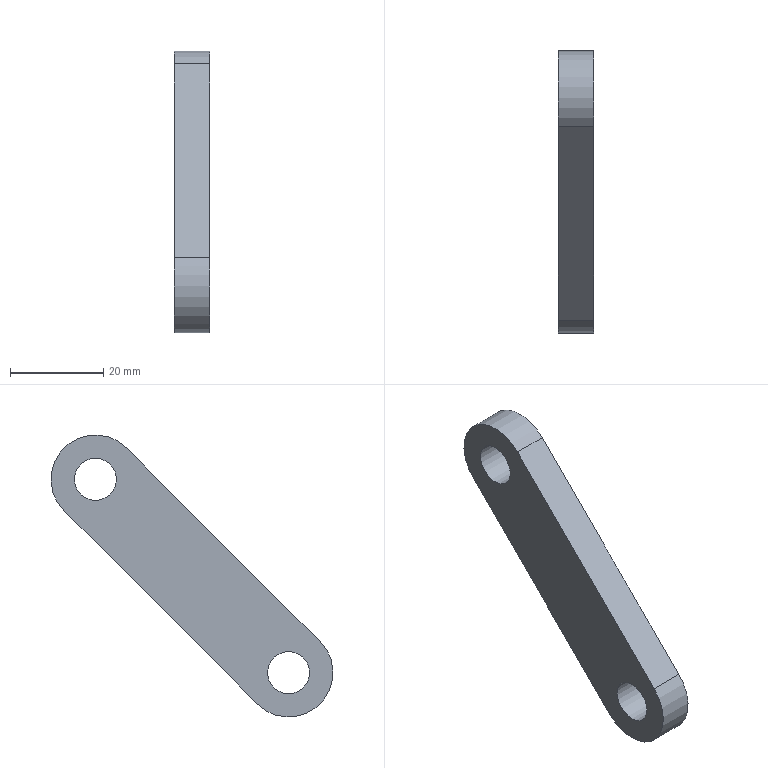Part | NX | features solid 2 | 1 solid | 8 faces | box 7.5 x 60.366 x 60.366 mm | volume 9508 mm3 | plane 4 | cylinder 4 | commonest cylinder face diameters 9 x2 19 x2
STEP:
#1=CARTESIAN_POINT('',(-28.5,179.948,172.083));
#2=VERTEX_POINT('',#1);
#3=CARTESIAN_POINT('',(-28.5,138.582,130.718));
#4=VERTEX_POINT('',#3);
#5=CARTESIAN_POINT('',(-28.5,133.279,125.414));
#6=DIRECTION('',(-0.000000007,-0.7071,-0.7071));
#7=VECTOR('',#6,1000.);
#8=LINE('',#5,#7);
#9=EDGE_CURVE('',#2,#4,#8,.T.);
#10=ORIENTED_EDGE('',*,*,#9,.T.);
#11=CARTESIAN_POINT('',(-21.,138.582,130.718));
#12=VERTEX_POINT('',#11);
#13=CARTESIAN_POINT('',(-24.75,138.582,130.718));
#14=DIRECTION('',(-1.,-0.000000003,0.000000012));
#15=VECTOR('',#14,1000.);
#16=LINE('',#13,#15);
#17=EDGE_CURVE('',#4,#12,#16,.F.);
#18=ORIENTED_EDGE('',*,*,#17,.T.);
#19=CARTESIAN_POINT('',(-21.,179.948,172.083));
#20=VERTEX_POINT('',#19);
#21=CARTESIAN_POINT('',(-21.,133.279,125.414));
#22=DIRECTION('',(-0.000000007,-0.7071,-0.7071));
#23=VECTOR('',#22,1000.);
#24=LINE('',#21,#23);
#25=EDGE_CURVE('',#20,#12,#24,.T.);
#26=ORIENTED_EDGE('',*,*,#25,.F.);
#27=CARTESIAN_POINT('',(-24.75,179.948,172.083));
#28=DIRECTION('',(1.,0.000000003,-0.000000012));
#29=VECTOR('',#28,1000.);
#30=LINE('',#27,#29);
#31=EDGE_CURVE('',#20,#2,#30,.F.);
#32=ORIENTED_EDGE('',*,*,#31,.T.);
#33=EDGE_LOOP('',(#10,#18,#26,#32));
#34=FACE_BOUND('',#33,.T.);
#35=CARTESIAN_POINT('',(-24.75,133.279,125.414));
#36=DIRECTION('',(0.000000011,-0.7071,0.7071));
#37=DIRECTION('',(-0.000000013,-0.7071,-0.7071));
#38=AXIS2_PLACEMENT_3D('',#35,#36,#37);
#39=PLANE('',#38);
#40=ADVANCED_FACE('',(#34),#39,.T.);
#41=CARTESIAN_POINT('',(-21.,186.666,169.866));
#42=VERTEX_POINT('',#41);
#43=CARTESIAN_POINT('',(-21.,186.666,165.366));
#44=DIRECTION('',(-1.,-0.000000003,0.000000012));
#45=DIRECTION('',(0.000000012,0.,1.));
#46=AXIS2_PLACEMENT_3D('',#43,#44,#45);
#47=CIRCLE('',#46,4.5);
#48=EDGE_CURVE('',#42,#42,#47,.F.);
#49=ORIENTED_EDGE('',*,*,#48,.F.);
#50=EDGE_LOOP('',(#49));
#51=FACE_BOUND('',#50,.T.);
#52=CARTESIAN_POINT('',(-21.,145.3,128.5));
#53=VERTEX_POINT('',#52);
#54=CARTESIAN_POINT('',(-21.,145.3,124.));
#55=DIRECTION('',(-1.,-0.000000003,0.000000012));
#56=DIRECTION('',(0.000000012,0.,1.));
#57=AXIS2_PLACEMENT_3D('',#54,#55,#56);
#58=CIRCLE('',#57,4.5);
#59=EDGE_CURVE('',#53,#53,#58,.F.);
#60=ORIENTED_EDGE('',*,*,#59,.F.);
#61=EDGE_LOOP('',(#60));
#62=FACE_BOUND('',#61,.T.);
#63=CARTESIAN_POINT('',(-21.,193.383,158.648));
#64=VERTEX_POINT('',#63);
#65=CARTESIAN_POINT('',(-21.,186.666,165.366));
#66=DIRECTION('',(1.,0.000000003,-0.000000012));
#67=DIRECTION('',(-0.000000012,0.,-1.));
#68=AXIS2_PLACEMENT_3D('',#65,#66,#67);
#69=CIRCLE('',#68,9.5);
#70=EDGE_CURVE('',#64,#20,#69,.T.);
#71=ORIENTED_EDGE('',*,*,#70,.T.);
#72=ORIENTED_EDGE('',*,*,#25,.T.);
#73=CARTESIAN_POINT('',(-21.,152.018,117.282));
#74=VERTEX_POINT('',#73);
#75=CARTESIAN_POINT('',(-21.,145.3,124.));
#76=DIRECTION('',(1.,0.000000003,-0.000000012));
#77=DIRECTION('',(-0.000000012,0.,-1.));
#78=AXIS2_PLACEMENT_3D('',#75,#76,#77);
#79=CIRCLE('',#78,9.5);
#80=EDGE_CURVE('',#12,#74,#79,.T.);
#81=ORIENTED_EDGE('',*,*,#80,.T.);
#82=CARTESIAN_POINT('',(-21.,146.714,111.979));
#83=DIRECTION('',(-0.000000007,-0.7071,-0.7071));
#84=VECTOR('',#83,1000.);
#85=LINE('',#82,#84);
#86=EDGE_CURVE('',#64,#74,#85,.T.);
#87=ORIENTED_EDGE('',*,*,#86,.F.);
#88=EDGE_LOOP('',(#71,#72,#81,#87));
#89=FACE_BOUND('',#88,.T.);
#90=CARTESIAN_POINT('',(-21.,139.997,118.697));
#91=DIRECTION('',(1.,0.000000003,-0.000000012));
#92=DIRECTION('',(0.000000012,0.,1.));
#93=AXIS2_PLACEMENT_3D('',#90,#91,#92);
#94=PLANE('',#93);
#95=ADVANCED_FACE('',(#51,#62,#89),#94,.T.);
#96=ORIENTED_EDGE('',*,*,#86,.T.);
#97=CARTESIAN_POINT('',(-28.5,152.018,117.282));
#98=VERTEX_POINT('',#97);
#99=CARTESIAN_POINT('',(-24.75,152.018,117.282));
#100=DIRECTION('',(-1.,-0.000000003,0.000000012));
#101=VECTOR('',#100,1000.);
#102=LINE('',#99,#101);
#103=EDGE_CURVE('',#74,#98,#102,.T.);
#104=ORIENTED_EDGE('',*,*,#103,.T.);
#105=CARTESIAN_POINT('',(-28.5,193.383,158.648));
#106=VERTEX_POINT('',#105);
#107=CARTESIAN_POINT('',(-28.5,146.714,111.979));
#108=DIRECTION('',(-0.000000007,-0.7071,-0.7071));
#109=VECTOR('',#108,1000.);
#110=LINE('',#107,#109);
#111=EDGE_CURVE('',#106,#98,#110,.T.);
#112=ORIENTED_EDGE('',*,*,#111,.F.);
#113=CARTESIAN_POINT('',(-24.75,193.383,158.648));
#114=DIRECTION('',(1.,0.000000003,-0.000000012));
#115=VECTOR('',#114,1000.);
#116=LINE('',#113,#115);
#117=EDGE_CURVE('',#106,#64,#116,.T.);
#118=ORIENTED_EDGE('',*,*,#117,.T.);
#119=EDGE_LOOP('',(#96,#104,#112,#118));
#120=FACE_BOUND('',#119,.T.);
#121=CARTESIAN_POINT('',(-24.75,146.714,111.979));
#122=DIRECTION('',(-0.000000011,0.7071,-0.7071));
#123=DIRECTION('',(0.000000013,0.7071,0.7071));
#124=AXIS2_PLACEMENT_3D('',#121,#122,#123);
#125=PLANE('',#124);
#126=ADVANCED_FACE('',(#120),#125,.T.);
#127=CARTESIAN_POINT('',(-28.5,186.666,169.866));
#128=VERTEX_POINT('',#127);
#129=CARTESIAN_POINT('',(-28.5,186.666,165.366));
#130=DIRECTION('',(-1.,-0.000000003,0.000000012));
#131=DIRECTION('',(0.000000012,0.,1.));
#132=AXIS2_PLACEMENT_3D('',#129,#130,#131);
#133=CIRCLE('',#132,4.5);
#134=EDGE_CURVE('',#128,#128,#133,.F.);
#135=ORIENTED_EDGE('',*,*,#134,.T.);
#136=EDGE_LOOP('',(#135));
#137=FACE_BOUND('',#136,.T.);
#138=CARTESIAN_POINT('',(-28.5,145.3,128.5));
#139=VERTEX_POINT('',#138);
#140=CARTESIAN_POINT('',(-28.5,145.3,124.));
#141=DIRECTION('',(-1.,-0.000000003,0.000000012));
#142=DIRECTION('',(0.000000012,0.,1.));
#143=AXIS2_PLACEMENT_3D('',#140,#141,#142);
#144=CIRCLE('',#143,4.5);
#145=EDGE_CURVE('',#139,#139,#144,.F.);
#146=ORIENTED_EDGE('',*,*,#145,.T.);
#147=EDGE_LOOP('',(#146));
#148=FACE_BOUND('',#147,.T.);
#149=ORIENTED_EDGE('',*,*,#111,.T.);
#150=CARTESIAN_POINT('',(-28.5,145.3,124.));
#151=DIRECTION('',(-1.,-0.000000003,0.000000012));
#152=DIRECTION('',(0.000000012,0.,1.));
#153=AXIS2_PLACEMENT_3D('',#150,#151,#152);
#154=CIRCLE('',#153,9.5);
#155=EDGE_CURVE('',#98,#4,#154,.T.);
#156=ORIENTED_EDGE('',*,*,#155,.T.);
#157=ORIENTED_EDGE('',*,*,#9,.F.);
#158=CARTESIAN_POINT('',(-28.5,186.666,165.366));
#159=DIRECTION('',(-1.,-0.000000003,0.000000012));
#160=DIRECTION('',(0.000000012,0.,1.));
#161=AXIS2_PLACEMENT_3D('',#158,#159,#160);
#162=CIRCLE('',#161,9.5);
#163=EDGE_CURVE('',#2,#106,#162,.T.);
#164=ORIENTED_EDGE('',*,*,#163,.T.);
#165=EDGE_LOOP('',(#149,#156,#157,#164));
#166=FACE_BOUND('',#165,.T.);
#167=CARTESIAN_POINT('',(-28.5,139.997,118.697));
#168=DIRECTION('',(-1.,-0.000000003,0.000000012));
#169=DIRECTION('',(-0.000000012,0.,-1.));
#170=AXIS2_PLACEMENT_3D('',#167,#168,#169);
#171=PLANE('',#170);
#172=ADVANCED_FACE('',(#137,#148,#166),#171,.T.);
#173=ORIENTED_EDGE('',*,*,#80,.F.);
#174=ORIENTED_EDGE('',*,*,#17,.F.);
#175=ORIENTED_EDGE('',*,*,#155,.F.);
#176=ORIENTED_EDGE('',*,*,#103,.F.);
#177=EDGE_LOOP('',(#173,#174,#175,#176));
#178=FACE_BOUND('',#177,.T.);
#179=CARTESIAN_POINT('',(-24.75,145.3,124.));
#180=DIRECTION('',(-1.,-0.000000003,0.000000012));
#181=DIRECTION('',(-0.000000012,0.,-1.));
#182=AXIS2_PLACEMENT_3D('',#179,#180,#181);
#183=CYLINDRICAL_SURFACE('',#182,9.5);
#184=ADVANCED_FACE('',(#178),#183,.T.);
#185=ORIENTED_EDGE('',*,*,#163,.F.);
#186=ORIENTED_EDGE('',*,*,#31,.F.);
#187=ORIENTED_EDGE('',*,*,#70,.F.);
#188=ORIENTED_EDGE('',*,*,#117,.F.);
#189=EDGE_LOOP('',(#185,#186,#187,#188));
#190=FACE_BOUND('',#189,.T.);
#191=CARTESIAN_POINT('',(-24.75,186.666,165.366));
#192=DIRECTION('',(1.,0.000000003,-0.000000012));
#193=DIRECTION('',(0.000000012,0.,1.));
#194=AXIS2_PLACEMENT_3D('',#191,#192,#193);
#195=CYLINDRICAL_SURFACE('',#194,9.5);
#196=ADVANCED_FACE('',(#190),#195,.T.);
#197=ORIENTED_EDGE('',*,*,#59,.T.);
#198=EDGE_LOOP('',(#197));
#199=FACE_BOUND('',#198,.T.);
#200=ORIENTED_EDGE('',*,*,#145,.F.);
#201=EDGE_LOOP('',(#200));
#202=FACE_BOUND('',#201,.T.);
#203=CARTESIAN_POINT('',(-28.5,145.3,124.));
#204=DIRECTION('',(1.,0.000000003,-0.000000012));
#205=DIRECTION('',(0.000000012,0.,1.));
#206=AXIS2_PLACEMENT_3D('',#203,#204,#205);
#207=CYLINDRICAL_SURFACE('',#206,4.5);
#208=ADVANCED_FACE('',(#199,#202),#207,.F.);
#209=ORIENTED_EDGE('',*,*,#48,.T.);
#210=EDGE_LOOP('',(#209));
#211=FACE_BOUND('',#210,.T.);
#212=ORIENTED_EDGE('',*,*,#134,.F.);
#213=EDGE_LOOP('',(#212));
#214=FACE_BOUND('',#213,.T.);
#215=CARTESIAN_POINT('',(-28.5,186.666,165.366));
#216=DIRECTION('',(1.,0.000000003,-0.000000012));
#217=DIRECTION('',(0.000000012,0.,1.));
#218=AXIS2_PLACEMENT_3D('',#215,#216,#217);
#219=CYLINDRICAL_SURFACE('',#218,4.5);
#220=ADVANCED_FACE('',(#211,#214),#219,.F.);
#221=CLOSED_SHELL('',(#40,#95,#126,#172,#184,#196,#208,#220));
#222=MANIFOLD_SOLID_BREP('',#221);
#223=(LENGTH_UNIT()NAMED_UNIT(*)SI_UNIT(.MILLI.,.METRE.));
#224=UNCERTAINTY_MEASURE_WITH_UNIT(LENGTH_MEASURE(0.00001),#223,'','');
#225=(NAMED_UNIT(*)PLANE_ANGLE_UNIT()SI_UNIT($,.RADIAN.));
#226=(NAMED_UNIT(*)SI_UNIT($,.STERADIAN.)SOLID_ANGLE_UNIT());
#227=(GEOMETRIC_REPRESENTATION_CONTEXT(3)GLOBAL_UNCERTAINTY_ASSIGNED_CONTEXT((#224))GLOBAL_UNIT_ASSIGNED_CONTEXT((#223,#225,#226))REPRESENTATION_CONTEXT('',''));
#228=ADVANCED_BREP_SHAPE_REPRESENTATION('',(#222),#227);